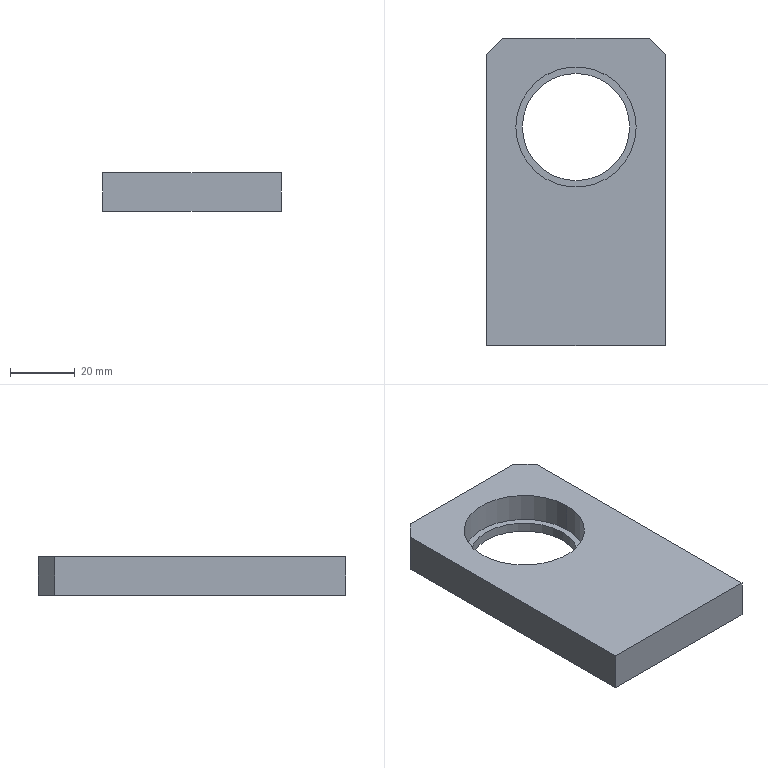Part | SolidWorks | features ICE 4, Chamfer 1, Extrusion 1 | 1 solid | 13 faces | box 55 x 94.5 x 12 mm | volume 49827 mm3 | plane 9 | cylinder 4 | commonest cylinder face diameters 33 x2 37 x2
STEP:
#1=CARTESIAN_POINT('',(16.5,20.,3.));
#2=VERTEX_POINT('',#1);
#3=CARTESIAN_POINT('',(-16.5,20.,3.));
#4=VERTEX_POINT('',#3);
#5=CARTESIAN_POINT('',(0.,20.,3.));
#6=DIRECTION('',(0.,0.,-1.));
#7=DIRECTION('',(-1.,0.,0.));
#8=AXIS2_PLACEMENT_3D('',#5,#6,#7);
#9=CIRCLE('',#8,16.5);
#10=EDGE_CURVE('',#2,#4,#9,.T.);
#11=ORIENTED_EDGE('',*,*,#10,.F.);
#12=CARTESIAN_POINT('',(16.5,20.,0.));
#13=VERTEX_POINT('',#12);
#14=CARTESIAN_POINT('',(16.5,20.,3.));
#15=DIRECTION('',(0.,0.,-1.));
#16=VECTOR('',#15,1000.);
#17=LINE('',#14,#16);
#18=EDGE_CURVE('',#2,#13,#17,.T.);
#19=ORIENTED_EDGE('',*,*,#18,.T.);
#20=CARTESIAN_POINT('',(-16.5,20.,0.));
#21=VERTEX_POINT('',#20);
#22=CARTESIAN_POINT('',(0.,20.,0.));
#23=DIRECTION('',(0.,0.,-1.));
#24=DIRECTION('',(-1.,0.,0.));
#25=AXIS2_PLACEMENT_3D('',#22,#23,#24);
#26=CIRCLE('',#25,16.5);
#27=EDGE_CURVE('',#13,#21,#26,.T.);
#28=ORIENTED_EDGE('',*,*,#27,.T.);
#29=CARTESIAN_POINT('',(-16.5,20.,3.));
#30=DIRECTION('',(0.,0.,-1.));
#31=VECTOR('',#30,1000.);
#32=LINE('',#29,#31);
#33=EDGE_CURVE('',#4,#21,#32,.T.);
#34=ORIENTED_EDGE('',*,*,#33,.F.);
#35=EDGE_LOOP('',(#11,#19,#28,#34));
#36=FACE_OUTER_BOUND('',#35,.T.);
#37=CARTESIAN_POINT('',(0.,20.,3.));
#38=DIRECTION('',(0.,0.,-1.));
#39=DIRECTION('',(-1.,0.,0.));
#40=AXIS2_PLACEMENT_3D('',#37,#38,#39);
#41=CYLINDRICAL_SURFACE('',#40,16.5);
#42=ADVANCED_FACE('',(#36),#41,.F.);
#43=CARTESIAN_POINT('',(-18.5,20.,12.));
#44=VERTEX_POINT('',#43);
#45=CARTESIAN_POINT('',(18.5,20.,12.));
#46=VERTEX_POINT('',#45);
#47=CARTESIAN_POINT('',(0.,20.,12.));
#48=DIRECTION('',(0.,0.,1.));
#49=DIRECTION('',(-1.,0.,0.));
#50=AXIS2_PLACEMENT_3D('',#47,#48,#49);
#51=CIRCLE('',#50,18.5);
#52=EDGE_CURVE('',#44,#46,#51,.T.);
#53=ORIENTED_EDGE('',*,*,#52,.T.);
#54=CARTESIAN_POINT('',(18.5,20.,3.));
#55=VERTEX_POINT('',#54);
#56=CARTESIAN_POINT('',(18.5,20.,12.001));
#57=DIRECTION('',(0.,0.,-1.));
#58=VECTOR('',#57,1000.);
#59=LINE('',#56,#58);
#60=EDGE_CURVE('',#46,#55,#59,.T.);
#61=ORIENTED_EDGE('',*,*,#60,.T.);
#62=CARTESIAN_POINT('',(-18.5,20.,3.));
#63=VERTEX_POINT('',#62);
#64=CARTESIAN_POINT('',(0.,20.,3.));
#65=DIRECTION('',(0.,0.,1.));
#66=DIRECTION('',(-1.,0.,0.));
#67=AXIS2_PLACEMENT_3D('',#64,#65,#66);
#68=CIRCLE('',#67,18.5);
#69=EDGE_CURVE('',#63,#55,#68,.T.);
#70=ORIENTED_EDGE('',*,*,#69,.F.);
#71=CARTESIAN_POINT('',(-18.5,20.,12.001));
#72=DIRECTION('',(0.,0.,-1.));
#73=VECTOR('',#72,1000.);
#74=LINE('',#71,#73);
#75=EDGE_CURVE('',#44,#63,#74,.T.);
#76=ORIENTED_EDGE('',*,*,#75,.F.);
#77=EDGE_LOOP('',(#53,#61,#70,#76));
#78=FACE_OUTER_BOUND('',#77,.T.);
#79=CARTESIAN_POINT('',(0.,20.,12.001));
#80=DIRECTION('',(0.,0.,-1.));
#81=DIRECTION('',(-1.,0.,0.));
#82=AXIS2_PLACEMENT_3D('',#79,#80,#81);
#83=CYLINDRICAL_SURFACE('',#82,18.5);
#84=ADVANCED_FACE('',(#78),#83,.F.);
#85=ORIENTED_EDGE('',*,*,#60,.F.);
#86=CARTESIAN_POINT('',(0.,20.,12.));
#87=DIRECTION('',(0.,0.,1.));
#88=DIRECTION('',(-1.,0.,0.));
#89=AXIS2_PLACEMENT_3D('',#86,#87,#88);
#90=CIRCLE('',#89,18.5);
#91=EDGE_CURVE('',#46,#44,#90,.T.);
#92=ORIENTED_EDGE('',*,*,#91,.T.);
#93=ORIENTED_EDGE('',*,*,#75,.T.);
#94=CARTESIAN_POINT('',(0.,20.,3.));
#95=DIRECTION('',(0.,0.,1.));
#96=DIRECTION('',(-1.,0.,0.));
#97=AXIS2_PLACEMENT_3D('',#94,#95,#96);
#98=CIRCLE('',#97,18.5);
#99=EDGE_CURVE('',#55,#63,#98,.T.);
#100=ORIENTED_EDGE('',*,*,#99,.F.);
#101=EDGE_LOOP('',(#85,#92,#93,#100));
#102=FACE_OUTER_BOUND('',#101,.T.);
#103=CARTESIAN_POINT('',(0.,20.,12.001));
#104=DIRECTION('',(0.,0.,-1.));
#105=DIRECTION('',(-1.,0.,0.));
#106=AXIS2_PLACEMENT_3D('',#103,#104,#105);
#107=CYLINDRICAL_SURFACE('',#106,18.5);
#108=ADVANCED_FACE('',(#102),#107,.F.);
#109=CARTESIAN_POINT('',(27.5,-47.25,0.));
#110=VERTEX_POINT('',#109);
#111=CARTESIAN_POINT('',(27.5,42.25,0.));
#112=VERTEX_POINT('',#111);
#113=CARTESIAN_POINT('',(27.5,-47.25,0.));
#114=DIRECTION('',(0.,1.,0.));
#115=VECTOR('',#114,1000.);
#116=LINE('',#113,#115);
#117=EDGE_CURVE('',#110,#112,#116,.T.);
#118=ORIENTED_EDGE('',*,*,#117,.T.);
#119=CARTESIAN_POINT('',(27.5,42.25,12.));
#120=VERTEX_POINT('',#119);
#121=CARTESIAN_POINT('',(27.5,42.25,12.));
#122=DIRECTION('',(0.,0.,1.));
#123=VECTOR('',#122,1000.);
#124=LINE('',#121,#123);
#125=EDGE_CURVE('',#112,#120,#124,.T.);
#126=ORIENTED_EDGE('',*,*,#125,.T.);
#127=CARTESIAN_POINT('',(27.5,-47.25,12.));
#128=VERTEX_POINT('',#127);
#129=CARTESIAN_POINT('',(27.5,-47.25,12.));
#130=DIRECTION('',(0.,1.,0.));
#131=VECTOR('',#130,1000.);
#132=LINE('',#129,#131);
#133=EDGE_CURVE('',#128,#120,#132,.T.);
#134=ORIENTED_EDGE('',*,*,#133,.F.);
#135=CARTESIAN_POINT('',(27.5,-47.25,12.));
#136=DIRECTION('',(0.,0.,-1.));
#137=VECTOR('',#136,1000.);
#138=LINE('',#135,#137);
#139=EDGE_CURVE('',#128,#110,#138,.T.);
#140=ORIENTED_EDGE('',*,*,#139,.T.);
#141=EDGE_LOOP('',(#118,#126,#134,#140));
#142=FACE_OUTER_BOUND('',#141,.T.);
#143=CARTESIAN_POINT('',(27.5,-47.25,12.));
#144=DIRECTION('',(-1.,0.,0.));
#145=DIRECTION('',(0.,0.,1.));
#146=AXIS2_PLACEMENT_3D('',#143,#144,#145);
#147=PLANE('',#146);
#148=ADVANCED_FACE('',(#142),#147,.F.);
#149=CARTESIAN_POINT('',(22.5,47.25,0.));
#150=VERTEX_POINT('',#149);
#151=CARTESIAN_POINT('',(-22.5,47.25,0.));
#152=VERTEX_POINT('',#151);
#153=CARTESIAN_POINT('',(-27.5,47.25,0.));
#154=DIRECTION('',(-1.,0.,0.));
#155=VECTOR('',#154,1000.);
#156=LINE('',#153,#155);
#157=EDGE_CURVE('',#150,#152,#156,.T.);
#158=ORIENTED_EDGE('',*,*,#157,.T.);
#159=CARTESIAN_POINT('',(-22.5,47.25,12.));
#160=VERTEX_POINT('',#159);
#161=CARTESIAN_POINT('',(-22.5,47.25,12.));
#162=DIRECTION('',(0.,0.,1.));
#163=VECTOR('',#162,1000.);
#164=LINE('',#161,#163);
#165=EDGE_CURVE('',#152,#160,#164,.T.);
#166=ORIENTED_EDGE('',*,*,#165,.T.);
#167=CARTESIAN_POINT('',(22.5,47.25,12.));
#168=VERTEX_POINT('',#167);
#169=CARTESIAN_POINT('',(-27.5,47.25,12.));
#170=DIRECTION('',(-1.,0.,0.));
#171=VECTOR('',#170,1000.);
#172=LINE('',#169,#171);
#173=EDGE_CURVE('',#168,#160,#172,.T.);
#174=ORIENTED_EDGE('',*,*,#173,.F.);
#175=CARTESIAN_POINT('',(22.5,47.25,12.));
#176=DIRECTION('',(0.,0.,-1.));
#177=VECTOR('',#176,1000.);
#178=LINE('',#175,#177);
#179=EDGE_CURVE('',#168,#150,#178,.T.);
#180=ORIENTED_EDGE('',*,*,#179,.T.);
#181=EDGE_LOOP('',(#158,#166,#174,#180));
#182=FACE_OUTER_BOUND('',#181,.T.);
#183=CARTESIAN_POINT('',(-27.5,47.25,12.));
#184=DIRECTION('',(0.,-1.,0.));
#185=DIRECTION('',(0.,0.,-1.));
#186=AXIS2_PLACEMENT_3D('',#183,#184,#185);
#187=PLANE('',#186);
#188=ADVANCED_FACE('',(#182),#187,.F.);
#189=CARTESIAN_POINT('',(-27.5,42.25,12.));
#190=VERTEX_POINT('',#189);
#191=CARTESIAN_POINT('',(-27.5,-47.25,12.));
#192=VERTEX_POINT('',#191);
#193=CARTESIAN_POINT('',(-27.5,-47.25,12.));
#194=DIRECTION('',(0.,-1.,0.));
#195=VECTOR('',#194,1000.);
#196=LINE('',#193,#195);
#197=EDGE_CURVE('',#190,#192,#196,.T.);
#198=ORIENTED_EDGE('',*,*,#197,.F.);
#199=CARTESIAN_POINT('',(-27.5,42.25,0.));
#200=VERTEX_POINT('',#199);
#201=CARTESIAN_POINT('',(-27.5,42.25,12.));
#202=DIRECTION('',(0.,0.,-1.));
#203=VECTOR('',#202,1000.);
#204=LINE('',#201,#203);
#205=EDGE_CURVE('',#190,#200,#204,.T.);
#206=ORIENTED_EDGE('',*,*,#205,.T.);
#207=CARTESIAN_POINT('',(-27.5,-47.25,0.));
#208=VERTEX_POINT('',#207);
#209=CARTESIAN_POINT('',(-27.5,-47.25,0.));
#210=DIRECTION('',(0.,-1.,0.));
#211=VECTOR('',#210,1000.);
#212=LINE('',#209,#211);
#213=EDGE_CURVE('',#200,#208,#212,.T.);
#214=ORIENTED_EDGE('',*,*,#213,.T.);
#215=CARTESIAN_POINT('',(-27.5,-47.25,12.));
#216=DIRECTION('',(0.,0.,-1.));
#217=VECTOR('',#216,1000.);
#218=LINE('',#215,#217);
#219=EDGE_CURVE('',#192,#208,#218,.T.);
#220=ORIENTED_EDGE('',*,*,#219,.F.);
#221=EDGE_LOOP('',(#198,#206,#214,#220));
#222=FACE_OUTER_BOUND('',#221,.T.);
#223=CARTESIAN_POINT('',(-27.5,-47.25,12.));
#224=DIRECTION('',(1.,0.,0.));
#225=DIRECTION('',(0.,0.,-1.));
#226=AXIS2_PLACEMENT_3D('',#223,#224,#225);
#227=PLANE('',#226);
#228=ADVANCED_FACE('',(#222),#227,.F.);
#229=CARTESIAN_POINT('',(-27.5,-47.25,0.));
#230=DIRECTION('',(1.,0.,0.));
#231=VECTOR('',#230,1000.);
#232=LINE('',#229,#231);
#233=EDGE_CURVE('',#208,#110,#232,.T.);
#234=ORIENTED_EDGE('',*,*,#233,.T.);
#235=ORIENTED_EDGE('',*,*,#139,.F.);
#236=CARTESIAN_POINT('',(-27.5,-47.25,12.));
#237=DIRECTION('',(1.,0.,0.));
#238=VECTOR('',#237,1000.);
#239=LINE('',#236,#238);
#240=EDGE_CURVE('',#192,#128,#239,.T.);
#241=ORIENTED_EDGE('',*,*,#240,.F.);
#242=ORIENTED_EDGE('',*,*,#219,.T.);
#243=EDGE_LOOP('',(#234,#235,#241,#242));
#244=FACE_OUTER_BOUND('',#243,.T.);
#245=CARTESIAN_POINT('',(-27.5,-47.25,12.));
#246=DIRECTION('',(0.,1.,0.));
#247=DIRECTION('',(0.,0.,1.));
#248=AXIS2_PLACEMENT_3D('',#245,#246,#247);
#249=PLANE('',#248);
#250=ADVANCED_FACE('',(#244),#249,.F.);
#251=ORIENTED_EDGE('',*,*,#52,.F.);
#252=ORIENTED_EDGE('',*,*,#91,.F.);
#253=EDGE_LOOP('',(#251,#252));
#254=FACE_BOUND('',#253,.T.);
#255=ORIENTED_EDGE('',*,*,#173,.T.);
#256=CARTESIAN_POINT('',(-27.5,42.25,12.));
#257=DIRECTION('',(-0.7071,-0.7071,0.));
#258=VECTOR('',#257,1000.);
#259=LINE('',#256,#258);
#260=EDGE_CURVE('',#160,#190,#259,.T.);
#261=ORIENTED_EDGE('',*,*,#260,.T.);
#262=ORIENTED_EDGE('',*,*,#197,.T.);
#263=ORIENTED_EDGE('',*,*,#240,.T.);
#264=ORIENTED_EDGE('',*,*,#133,.T.);
#265=CARTESIAN_POINT('',(22.5,47.25,12.));
#266=DIRECTION('',(-0.7071,0.7071,0.));
#267=VECTOR('',#266,1000.);
#268=LINE('',#265,#267);
#269=EDGE_CURVE('',#120,#168,#268,.T.);
#270=ORIENTED_EDGE('',*,*,#269,.T.);
#271=EDGE_LOOP('',(#255,#261,#262,#263,#264,#270));
#272=FACE_OUTER_BOUND('',#271,.T.);
#273=CARTESIAN_POINT('',(0.,0.,12.));
#274=DIRECTION('',(0.,0.,-1.));
#275=DIRECTION('',(-1.,0.,0.));
#276=AXIS2_PLACEMENT_3D('',#273,#274,#275);
#277=PLANE('',#276);
#278=ADVANCED_FACE('',(#254,#272),#277,.F.);
#279=ORIENTED_EDGE('',*,*,#213,.F.);
#280=CARTESIAN_POINT('',(-34.875,34.875,0.));
#281=DIRECTION('',(0.7071,0.7071,0.));
#282=VECTOR('',#281,1000.);
#283=LINE('',#280,#282);
#284=EDGE_CURVE('',#200,#152,#283,.T.);
#285=ORIENTED_EDGE('',*,*,#284,.T.);
#286=ORIENTED_EDGE('',*,*,#157,.F.);
#287=CARTESIAN_POINT('',(34.875,34.875,0.));
#288=DIRECTION('',(0.7071,-0.7071,0.));
#289=VECTOR('',#288,1000.);
#290=LINE('',#287,#289);
#291=EDGE_CURVE('',#150,#112,#290,.T.);
#292=ORIENTED_EDGE('',*,*,#291,.T.);
#293=ORIENTED_EDGE('',*,*,#117,.F.);
#294=ORIENTED_EDGE('',*,*,#233,.F.);
#295=EDGE_LOOP('',(#279,#285,#286,#292,#293,#294));
#296=FACE_OUTER_BOUND('',#295,.T.);
#297=CARTESIAN_POINT('',(0.,20.,0.));
#298=DIRECTION('',(0.,0.,-1.));
#299=DIRECTION('',(-1.,0.,0.));
#300=AXIS2_PLACEMENT_3D('',#297,#298,#299);
#301=CIRCLE('',#300,16.5);
#302=EDGE_CURVE('',#21,#13,#301,.T.);
#303=ORIENTED_EDGE('',*,*,#302,.F.);
#304=ORIENTED_EDGE('',*,*,#27,.F.);
#305=EDGE_LOOP('',(#303,#304));
#306=FACE_BOUND('',#305,.T.);
#307=CARTESIAN_POINT('',(0.,0.,0.));
#308=DIRECTION('',(0.,0.,-1.));
#309=DIRECTION('',(-1.,0.,0.));
#310=AXIS2_PLACEMENT_3D('',#307,#308,#309);
#311=PLANE('',#310);
#312=ADVANCED_FACE('',(#296,#306),#311,.T.);
#313=ORIENTED_EDGE('',*,*,#260,.F.);
#314=ORIENTED_EDGE('',*,*,#165,.F.);
#315=ORIENTED_EDGE('',*,*,#284,.F.);
#316=ORIENTED_EDGE('',*,*,#205,.F.);
#317=EDGE_LOOP('',(#313,#314,#315,#316));
#318=FACE_OUTER_BOUND('',#317,.T.);
#319=CARTESIAN_POINT('',(-27.5,42.25,12.));
#320=DIRECTION('',(0.7071,-0.7071,0.));
#321=DIRECTION('',(0.,0.,-1.));
#322=AXIS2_PLACEMENT_3D('',#319,#320,#321);
#323=PLANE('',#322);
#324=ADVANCED_FACE('',(#318),#323,.F.);
#325=ORIENTED_EDGE('',*,*,#269,.F.);
#326=ORIENTED_EDGE('',*,*,#125,.F.);
#327=ORIENTED_EDGE('',*,*,#291,.F.);
#328=ORIENTED_EDGE('',*,*,#179,.F.);
#329=EDGE_LOOP('',(#325,#326,#327,#328));
#330=FACE_OUTER_BOUND('',#329,.T.);
#331=CARTESIAN_POINT('',(22.5,47.25,12.));
#332=DIRECTION('',(-0.7071,-0.7071,0.));
#333=DIRECTION('',(0.,0.,-1.));
#334=AXIS2_PLACEMENT_3D('',#331,#332,#333);
#335=PLANE('',#334);
#336=ADVANCED_FACE('',(#330),#335,.F.);
#337=CARTESIAN_POINT('',(0.,20.,3.));
#338=DIRECTION('',(0.,0.,-1.));
#339=DIRECTION('',(-1.,0.,0.));
#340=AXIS2_PLACEMENT_3D('',#337,#338,#339);
#341=CIRCLE('',#340,16.5);
#342=EDGE_CURVE('',#4,#2,#341,.T.);
#343=ORIENTED_EDGE('',*,*,#342,.T.);
#344=ORIENTED_EDGE('',*,*,#10,.T.);
#345=EDGE_LOOP('',(#343,#344));
#346=FACE_BOUND('',#345,.T.);
#347=ORIENTED_EDGE('',*,*,#69,.T.);
#348=ORIENTED_EDGE('',*,*,#99,.T.);
#349=EDGE_LOOP('',(#347,#348));
#350=FACE_OUTER_BOUND('',#349,.T.);
#351=CARTESIAN_POINT('',(0.,20.,3.));
#352=DIRECTION('',(0.,0.,-1.));
#353=DIRECTION('',(-1.,0.,0.));
#354=AXIS2_PLACEMENT_3D('',#351,#352,#353);
#355=PLANE('',#354);
#356=ADVANCED_FACE('',(#346,#350),#355,.F.);
#357=ORIENTED_EDGE('',*,*,#18,.F.);
#358=ORIENTED_EDGE('',*,*,#342,.F.);
#359=ORIENTED_EDGE('',*,*,#33,.T.);
#360=ORIENTED_EDGE('',*,*,#302,.T.);
#361=EDGE_LOOP('',(#357,#358,#359,#360));
#362=FACE_OUTER_BOUND('',#361,.T.);
#363=CARTESIAN_POINT('',(0.,20.,3.));
#364=DIRECTION('',(0.,0.,-1.));
#365=DIRECTION('',(-1.,0.,0.));
#366=AXIS2_PLACEMENT_3D('',#363,#364,#365);
#367=CYLINDRICAL_SURFACE('',#366,16.5);
#368=ADVANCED_FACE('',(#362),#367,.F.);
#369=CLOSED_SHELL('',(#42,#84,#108,#148,#188,#228,#250,#278,#312,#324,#336,#356,#368));
#370=MANIFOLD_SOLID_BREP('',#369);
#371=CARTESIAN_POINT('',(0.,0.,0.));
#372=DIRECTION('',(0.,0.,1.));
#373=DIRECTION('',(1.,0.,0.));
#374=AXIS2_PLACEMENT_3D('',#371,#372,#373);
#375=(LENGTH_UNIT()NAMED_UNIT(*)SI_UNIT(.MILLI.,.METRE.));
#376=UNCERTAINTY_MEASURE_WITH_UNIT(LENGTH_MEASURE(0.00001),#375,'','');
#377=(NAMED_UNIT(*)PLANE_ANGLE_UNIT()SI_UNIT($,.RADIAN.));
#378=(NAMED_UNIT(*)SI_UNIT($,.STERADIAN.)SOLID_ANGLE_UNIT());
#379=(GEOMETRIC_REPRESENTATION_CONTEXT(3)GLOBAL_UNCERTAINTY_ASSIGNED_CONTEXT((#376))GLOBAL_UNIT_ASSIGNED_CONTEXT((#375,#377,#378))REPRESENTATION_CONTEXT('',''));
#380=ADVANCED_BREP_SHAPE_REPRESENTATION('',(#370,#374),#379);